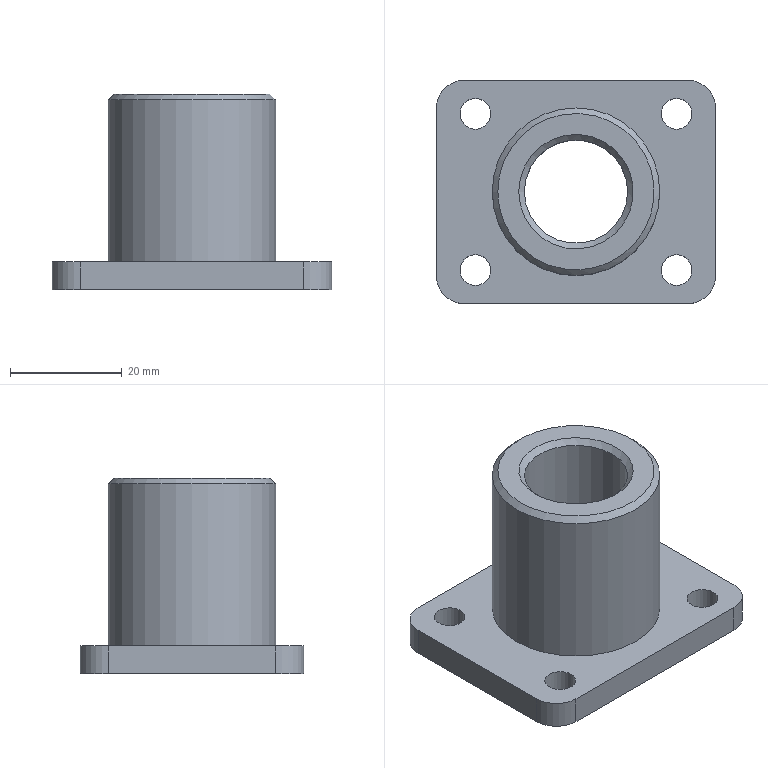NC program | NX | posted with a generic post | part box 50 x 40 x 35 mm
Whole program:
N10 G17 G21 G94 G90
(PLANAR_MILL , TOOL : D50面刀)
N12 T01 M6
N14 G53
N16 G17 G0 G90 X70. Y0. S3500 M3
N18 G43 Z20. H1
N20 Z3.
N22 G94 G1 Z0. F800.
N24 X20.
N26 X-20.
N28 X-70.
N30 Z3.
N32 G0 Z20.
N34 M5
(DRILLING , TOOL : D10倒角刀)
N36 T04 M6
N38 G53
N40 G17 G0 G90 X0. Y0. S1600 M3
N42 G43 Z20. H4
N44 G94 G81 G99 Z-2. F200. R3.
N46 G80
N48 G0 X0. Y0. Z20.
N50 M5
(DRILLING_COPY , TOOL : 14钻头)
N52 T06 M6
N54 G53
N56 G17 G0 G90 X0. Y0. S1600 M3
N58 G43 Z20. H6
N60 G94 G83 G99 Z-45. F250. Q3. R3.
N62 G80
N64 G0 X0. Y0. Z20.
N66 M5
(ADAPTIVE_MILLING , TOOL : D14开粗)
N68 T02 M6
N70 G53
N72 G17 G0 G90 X-43.532 Y-17.942 S6500 M3
N74 G43 Z20. H2
N76 Z-33.
N78 G94 G1 X-43.382 Y-17.95 Z-33.937 F2000.
N80 X-43.232 Y-17.957 Z-34.308
N82 X-43.082 Y-17.965 Z-34.58
N84 X-42.932 Y-17.972 Z-34.8
N86 X-42.783 Y-17.98 Z-34.984
N88 X-42.633 Y-17.987 Z-35.142
N90 X-42.483 Y-17.995 Z-35.28
N92 X-42.333 Y-18.002 Z-35.4
N94 X-42.183 Y-18.01 Z-35.505
N96 X-42.034 Y-18.017 Z-35.598
N98 X-41.884 Y-18.025 Z-35.679
N100 X-41.734 Y-18.032 Z-35.75
N102 X-41.584 Y-18.04 Z-35.81
N104 X-41.434 Y-18.047 Z-35.862
N106 X-41.284 Y-18.055 Z-35.905
N108 X-41.135 Y-18.062 Z-35.939
N110 X-40.985 Y-18.07 Z-35.966
N112 X-40.835 Y-18.077 Z-35.985
N114 X-40.685 Y-18.085 Z-35.996
N116 X-40.535 Y-18.092 Z-36.
N118 X-38.453 Y-18.196
N120 G3 X-37.016 Y-17.149 R1.414
N122 X-36.533 Y-13.375 R17.149
N124 X-36.401 Y-2.488 R270.705
N126 G1 X-36.399 Y22.214
N128 G2 X-33.919 Y27.676 R7.639
N130 X-28.648 Y30.469 R11.883
N132 X-22.412 Y31.271 R29.823
N134 X-10.623 Y31.399 R316.83
N136 G1 X27.261
N138 G2 X32.676 Y28.913 R7.655
N140 X35.469 Y23.637 R11.894
N142 X36.27 Y17.401 R29.853
N144 X36.398 Y5.657 R316.189
N146 G1 X36.4 Y-22.222
N148 G2 X33.984 Y-27.622 R7.616
N150 X28.819 Y-30.426 R11.696
N152 X22.677 Y-31.259 R28.633
N154 X12.059 Y-31.397 R260.732
N156 G1 X7.199 Y-31.4
N158 X-27.357 Y-31.398
N160 G2 X-32.715 Y-28.887 R7.676
N162 X-35.484 Y-23.601 R11.904
N164 X-36.072 Y-17.398 R21.042
N166 G3 X-35.801 Y-0.643 R380.067
N168 G1 X-35.8 Y19.424
N170 G2 X-31.703 Y27.393 R9.863
N172 X-25.709 Y29.964 R15.167
N174 X-18.51 Y30.696 R41.381
N176 X-3.436 Y30.8 R566.596
N178 G1 X24.503 Y30.799
N180 G2 X32.399 Y26.689 R9.871
N182 X34.958 Y20.73 R15.166
N184 X35.689 Y13.667 R40.664
N186 X35.799 Y-1.452 R535.868
N188 G1 X35.798 Y-19.567
N190 G2 X31.669 Y-27.422 R9.856
N192 X25.619 Y-29.984 R15.272
N194 X18.733 Y-30.688 R41.045
N196 X3.839 Y-30.799 R521.569
N198 G1 X-24.566 Y-30.798
N200 G2 X-32.451 Y-26.629 R9.868
N202 X-34.921 Y-20.358 R14.123
N204 X-35.279 Y-14.21 R39.912
N206 G1 X-35.204 Y-1.629
N208 X-35.201 Y2.819
N210 X-35.198 Y17.129
N212 G2 X-29.584 Y27.185 R11.38
N214 X-23.213 Y29.461 R18.218
N216 X-15.822 Y30.101 R51.205
N218 X-0.748 Y30.199 R632.596
N220 G1 X22.118 Y30.197
N222 G2 X32.12 Y24.685 R11.369
N224 X34.461 Y18.205 R18.106
N226 X35.1 Y10.814 R51.212
N228 X35.198 Y-3.765 R609.071
N230 G1 X35.197 Y-17.137
N232 G2 X29.715 Y-27.106 R11.346
N234 X23.371 Y-29.432 R17.945
N236 X15.803 Y-30.101 R50.392
N238 X0.728 Y-30.199 R636.552
N240 G1 X-22.137 Y-30.197
N242 G2 X-29.689 Y-27.53 R11.298
N244 X-33.537 Y-21.352 R13.017
N246 X-34.524 Y-14.782 R27.012
N248 X-34.619 Y-9.113 R151.751
N250 G1 X-34.613 Y11.532
N252 G2 X-34.531 Y16.689 R81.752
N254 X-28.342 Y26.506 R12.298
N256 X-21.572 Y28.845 R19.765
N258 X-13.326 Y29.509 R57.924
N260 X2.333 Y29.598 R787.319
N262 G1 X19.823 Y29.597
N264 G2 X25.174 Y28.771 R14.963
N266 X31.806 Y22.806 R12.578
N268 X33.943 Y15.962 R21.019
N270 X34.519 Y7.888 R64.124
N272 X34.598 Y-7.502 R831.686
N274 X34.564 Y-16.147 R327.966
N276 X28.33 Y-26.513 R12.319
N278 X21.544 Y-28.849 R19.837
N280 X13.658 Y-29.5 R56.548
N282 X-2.272 Y-29.598 R720.089
N284 G1 X-19.887 Y-29.597
N286 G2 X-25.275 Y-28.734 R14.703
N288 X-31.746 Y-22.661 R12.17
N290 X-33.576 Y-16.195 R20.188
N292 X-33.98 Y-8.83 R65.396
N294 G1 X-34.018 Y1.79
N296 G2 X-33.983 Y14.134 R697.678
N298 X-32.42 Y20.547 R14.428
N300 X-26.17 Y26.39 R13.695
N302 X-19.14 Y28.379 R23.417
N304 X-10.523 Y28.927 R74.411
N306 X4.867 Y28.998 R856.888
N308 G1 X17.797 Y28.997
N310 G2 X22.97 Y28.434 R19.245
N312 X30.83 Y22.215 R13.07
N314 X33.178 Y15.398 R20.771
N316 X33.878 Y7.425 R56.219
N318 X33.997 Y-8.054 R594.164
N320 X33.944 Y-14.753 R157.733
N322 X31.33 Y-22.25 R13.389
N324 X24.759 Y-26.999 R14.73
N326 X17.566 Y-28.567 R27.873
N328 X8.037 Y-28.962 R109.8
N330 G1 X-4.923 Y-28.998
N332 X-17.861 Y-28.996
N334 G2 X-23.031 Y-28.414 R18.708
N336 X-30.723 Y-22.081 R12.66
N338 X-32.828 Y-15.322 R20.451
N340 X-33.353 Y-7.515 R62.314
N342 X-33.387 Y12.505 R865.955
N344 X-32.16 Y18.645 R16.477
N346 X-29.105 Y23.006 R13.34
N348 G1 X-28.591 Y23.592
N350 X-27.396 Y24.64
N352 X-26.074 Y25.523
N354 X-24.649 Y26.225
N356 G2 X-17.453 Y27.846 R30.063
N358 X-7.75 Y28.344 R98.035
N360 X7.01 Y28.397 R895.492
N362 X17.76 Y28.363 R532.958
N364 X24.045 Y26.97 R15.784
N366 X27.947 Y24.157 R13.343
N368 G1 X28.592 Y23.591
N370 X29.64 Y22.396
N372 X30.523 Y21.074
N374 X31.225 Y19.649
N376 G2 X32.845 Y12.452 R30.107
N378 X33.339 Y3.019 R96.348
N380 X33.365 Y-12.68 R616.08
N382 X32.045 Y-18.888 R15.996
N384 X29.138 Y-22.968 R13.332
N386 G1 X28.591 Y-23.592
N388 X27.396 Y-24.64
N390 X26.074 Y-25.523
N392 X24.649 Y-26.225
N394 G2 X17.452 Y-27.845 R30.114
N396 X8.019 Y-28.339 R96.322
N398 X-7.011 Y-28.397 R888.753
N400 X-17.665 Y-28.366 R632.314
N402 X-23.661 Y-27.115 R15.692
N404 X-27.164 Y-24.795 R13.199
N406 G1 X-27.397 Y-24.639
N408 X-28.592 Y-23.591
N410 X-29.64 Y-22.396
N412 X-30.523 Y-21.074
N414 X-31.225 Y-19.649
N416 X-31.736 Y-18.144
N418 G2 X-32.417 Y-13.231 R34.125
N420 X-32.793 Y-2.44 R141.368
N422 X-32.796 Y11.145 R674.758
N424 X-32.076 Y16.121 R21.454
N426 G1 X-32.046 Y16.587
N428 X-31.736 Y18.146
N430 X-31.225 Y19.65
N432 X-30.522 Y21.076
N434 X-29.639 Y22.397
N436 X-28.591 Y23.592
N438 X-27.396 Y24.64
N440 X-26.074 Y25.523
N442 X-24.649 Y26.225
N444 X-23.144 Y26.736
N446 X-21.585 Y27.046
N448 G2 X-11.975 Y27.611 R540.608
N450 X3.953 Y27.795 R466.882
N452 X16.142 Y27.778 R845.082
N454 X21.076 Y27.079 R22.273
N456 G1 X21.587 Y27.046
N458 X23.146 Y26.736
N460 X24.65 Y26.225
N462 X26.076 Y25.522
N464 X27.397 Y24.639
N466 X27.972 Y24.134
N468 X27.397 Y24.639
N470 X26.076 Y25.522
N472 X24.65 Y26.225
N474 X23.146 Y26.736
N476 X21.587 Y27.046
N478 G3 X11.266 Y27.43 R117.228
N480 G1 X8.026 Y27.435
N482 X-16.089
N484 G2 X-17.302 Y28.138 R1.401
N486 X-17.235 Y29.638 Z-35.943 R1.408
N488 G1 X-16.551 Y30.616 Z-35.9
N490 X-16.015 Y31.382 F15000.
N492 G3 X-17.707 Y33.474 R1.4
N494 G1 X-18.122 Y33.301
N496 X-18.531 Y33.115
N498 G3 X-19.012 Y32.659 R1.417
N500 G1 X-20.324 Y30.628
N502 X-21.218 Y29.234 Z-35.96 F2000.
N504 G3 X-21.341 Y28.15 Z-36. R1.4
N506 X-20. Y27.15 R1.4
N508 G1 X20.
N510 X21.587 Y27.046
N512 X23.146 Y26.736
N514 X24.65 Y26.225
N516 X26.076 Y25.522
N518 X27.397 Y24.639
N520 X28.592 Y23.591
N522 X29.64 Y22.396
N524 X30.523 Y21.074
N526 X31.225 Y19.649
N528 X31.736 Y18.144
N530 X32.046 Y16.585
N532 G2 X32.612 Y6.926 R534.812
N534 X32.778 Y-11.037 R470.757
N536 X32.08 Y-16.061 R21.138
N538 G1 X32.046 Y-16.587
N540 X31.736 Y-18.146
N542 X31.225 Y-19.65
N544 X30.522 Y-21.076
N546 X29.639 Y-22.397
N548 X29.134 Y-22.972
N550 X29.639 Y-22.397
N552 X30.522 Y-21.076
N554 X31.225 Y-19.65
N556 X31.736 Y-18.146
N558 X32.046 Y-16.587
N560 G3 X32.422 Y-5.875 R116.901
N562 G1 X32.42 Y8.685
N564 X32.15 Y10.705
N566 Y15.
N568 Y-15.
N570 X32.046 Y-16.587
N572 X31.736 Y-18.146
N574 X31.225 Y-19.65
N576 X30.522 Y-21.076
N578 X29.639 Y-22.397
N580 X28.591 Y-23.592
N582 X27.396 Y-24.64
N584 X26.074 Y-25.523
N586 X24.649 Y-26.225
N588 X23.144 Y-26.736
N590 X21.585 Y-27.046
N592 G2 X12.052 Y-27.607 R563.562
N594 X-2.796 Y-27.793 R431.408
N596 X-16.045 Y-27.78 R944.863
N598 X-20.979 Y-27.086 R21.1
N600 G1 X-21.587 Y-27.046
N602 X-23.146 Y-26.736
N604 X-24.65 Y-26.225
N606 X-26.076 Y-25.522
N608 X-27.198 Y-24.772
N610 X-26.076 Y-25.522
N612 X-24.65 Y-26.225
N614 X-23.146 Y-26.736
N616 X-21.587 Y-27.046
N618 G3 X-11.191 Y-27.43 R117.669
N620 G1 X-7.771 Y-27.435
N622 X12.821 Y-27.433
N624 G2 X15.273 Y-27.15 R127.771
N626 G1 X20.
N628 X-20.
N630 X-21.587 Y-27.046
N632 X-23.146 Y-26.736
N634 X-24.65 Y-26.225
N636 X-26.076 Y-25.522
N638 X-27.397 Y-24.639
N640 X-28.592 Y-23.591
N642 X-29.64 Y-22.396
N644 X-30.523 Y-21.074
N646 X-31.225 Y-19.649
N648 X-31.736 Y-18.144
N650 X-32.046 Y-16.585
N652 X-32.15 Y-15.
N654 Y15.
N656 X-32.076 Y16.123
N658 G3 X-33.218 Y17.604 R1.414
N660 G1 X-35.305 Y18.008
N662 X-35.452 Y18.037 Z-35.996
N664 X-35.599 Y18.065 Z-35.985
N666 X-35.746 Y18.094 Z-35.966
N668 X-35.894 Y18.123 Z-35.939
N670 X-36.041 Y18.151 Z-35.905
N672 X-36.188 Y18.18 Z-35.862
N674 X-36.335 Y18.208 Z-35.81
N676 X-36.483 Y18.237 Z-35.75
N678 X-36.63 Y18.265 Z-35.679
N680 X-36.777 Y18.294 Z-35.598
N682 X-36.924 Y18.322 Z-35.505
N684 X-37.072 Y18.351 Z-35.4
N686 X-37.219 Y18.38 Z-35.28
N688 X-37.366 Y18.408 Z-35.142
N690 X-37.513 Y18.437 Z-34.984
N692 X-37.661 Y18.465 Z-34.8
N694 X-37.808 Y18.494 Z-34.58
N696 X-37.955 Y18.522 Z-34.308
N698 X-38.102 Y18.551 Z-33.937
N700 X-38.25 Y18.579 Z-33.
N702 G0 Z20.
N704 X-38.7 Y-6.809
N706 Z-26.85
N708 G1 X-38.55 Y-6.813 Z-27.787
N710 X-38.4 Y-6.817 Z-28.158
N712 X-38.25 Y-6.82 Z-28.43
N714 X-38.1 Y-6.824 Z-28.65
N716 X-37.95 Y-6.828 Z-28.834
N718 X-37.801 Y-6.831 Z-28.992
N720 X-37.651 Y-6.835 Z-29.13
N722 X-37.501 Y-6.839 Z-29.25
N724 X-37.351 Y-6.842 Z-29.355
N726 X-37.201 Y-6.846 Z-29.448
N728 X-37.051 Y-6.85 Z-29.529
N730 X-36.901 Y-6.853 Z-29.6
N732 X-36.751 Y-6.857 Z-29.66
N734 X-36.601 Y-6.861 Z-29.712
N736 X-36.451 Y-6.864 Z-29.755
N738 X-36.301 Y-6.868 Z-29.789
N740 X-36.151 Y-6.872 Z-29.816
N742 X-36.001 Y-6.876 Z-29.835
N744 X-35.851 Y-6.879 Z-29.846
N746 X-35.701 Y-6.883 Z-29.85
N748 X-33.567 Y-6.935
N750 G3 X-32.182 Y-5.94 R1.414
N752 X-31.703 Y-2.49 R15.204
N754 X-31.554 Y6.597 R197.471
N756 G2 X-31.507 Y13.923 R215.71
N758 X-29.004 Y21.222 R13.259
N760 X-22.352 Y25.589 R11.949
N762 X-16.389 Y26.402 R28.443
N764 X-5.68 Y26.547 R250.999
N766 G1 X-0.775 Y26.55
N768 X17.579 Y26.548
N770 G2 X23.737 Y25.432 R15.506
N772 X30.547 Y17.518 R11.813
N774 X31.405 Y11.381 R27.801
N776 X31.547 Y0.627 R256.51
N778 G1 X31.549 Y-12.328
N780 G2 X30.778 Y-17.827 R16.712
N782 X22.452 Y-25.562 R11.825
N784 X16.311 Y-26.406 R28.272
N786 X5.648 Y-26.547 R257.185
N788 G1 X0.788 Y-26.55
N790 X-17.522 Y-26.548
N792 G2 X-23.474 Y-25.54 R15.778
N794 X-30.563 Y-17.452 R11.817
N796 X-31.399 Y-11.447 R27.928
N798 X-31.276 Y-5.091 R43.192
N800 G3 X-30.958 Y7.369 R191.883
N802 G2 X-30.866 Y12.894 R85.759
N804 X-28.861 Y19.36 R13.812
N806 X-22.748 Y24.212 R12.536
N808 X-16.349 Y25.607 R23.605
N810 X-7.718 Y25.928 R103.177
N812 G1 X2.677 Y25.949
N814 X15.312 Y25.948
N816 G2 X20.716 Y25.415 R21.701
N818 X28.899 Y18.494 R12.045
N820 X30.534 Y12.065 R21.292
N822 X30.92 Y3.573 R85.532
N824 X30.92 Y-11.926 R744.474
N826 X29.606 Y-18.001 R15.514
N828 X23.265 Y-23.998 R12.141
N830 X16.947 Y-25.545 R21.872
N832 X8.453 Y-25.921 R87.79
N834 G1 X-2.436 Y-25.949
N836 X-15.307 Y-25.948
N838 G2 X-20.711 Y-25.416 R21.734
N840 X-28.932 Y-18.416 R12.054
N842 X-30.569 Y-11.66 R21.66
N844 X-30.631 Y-5.32 R49.027
N846 G3 X-30.339 Y9.899 R434.182
N848 G2 X-29.53 Y15.444 R18.973
N850 X-23.102 Y22.781 R12.665
N852 X-16.311 Y24.779 R21.244
N854 X-8.097 Y25.291 R69.757
N856 X4.773 Y25.349 R787.252
N858 X15.492 Y25.314 R544.392
N860 X21.172 Y24.264 R16.888
N862 X27.869 Y17.933 R12.755
N864 X29.794 Y11.211 R21.534
N866 X30.293 Y3.041 R70.958
N868 X30.31 Y-10.594 R418.892
N870 X29.175 Y-16.391 R16.492
N872 X22.814 Y-22.925 R12.802
N874 X16.032 Y-24.816 R21.962
N876 X7.635 Y-25.299 R75.047
N878 X-4.785 Y-25.349 R790.412
N880 X-15.487 Y-25.314 R545.573
N882 X-21.167 Y-24.266 R16.912
N884 X-27.876 Y-17.915 R12.753
N886 X-29.811 Y-10.513 R20.615
N888 X-29.93 Y-3.497 R66.222
N890 G3 X-29.735 Y8.839 R999.429
N892 G2 X-28.851 Y14.463 R18.936
N894 X-22.272 Y21.946 R13.339
N896 X-15.333 Y24.08 R21.918
N898 X-6.72 Y24.677 R67.673
N900 X13.962 Y24.716 R869.82
N902 X19.537 Y23.819 R18.458
N904 X26.954 Y17.259 R13.335
N906 X29.076 Y10.367 R21.88
N908 X29.679 Y1.664 R67.715
N910 X29.695 Y-9.45 R249.339
N912 X28.513 Y-15.33 R16.713
N914 X21.982 Y-22.094 R13.478
N916 X14.963 Y-24.134 R22.694
N918 X6.031 Y-24.691 R74.436
N920 X-13.957 Y-24.716 R893.754
N922 X-19.576 Y-23.806 R18.421
N924 X-27.034 Y-17.093 R13.335
N926 X-29.013 Y-9.969 R20.714
N928 X-29.269 Y-2.103 R66.869
N930 X-29.112 Y8.223 R463.309
N932 X-27.896 Y14.235 R17.553
N934 X-21.222 Y21.276 R14.033
N936 X-13.971 Y23.462 R23.238
N938 X-4.863 Y24.076 R72.374
N940 X12.596 Y24.114 R676.558
N942 X18.44 Y23.19 R19.381
N944 X26.213 Y16.341 R13.911
N946 X28.436 Y9.151 R22.843
N948 X29.062 Y0.585 R67.693
N950 X29.069 Y-8.503 R148.851
N952 X27.68 Y-14.701 R16.587
N954 X20.951 Y-21.41 R14.141
N956 X13.712 Y-23.499 R23.864
N958 X4.692 Y-24.08 R75.191
N960 X-12.768 Y-24.108 R606.454
N962 X-18.687 Y-23.102 R18.717
N964 X-26.389 Y-15.94 R13.855
N966 X-28.312 Y-8.756 R22.18
N968 X-28.625 Y-0.532 R73.519
N970 X-28.488 Y7.476 R161.926
N972 X-26.951 Y13.914 R17.178
N974 X-20.04 Y20.708 R14.713
N976 X-12.638 Y22.857 R24.676
N978 X-3.529 Y23.467 R75.35
N980 X11.455 Y23.506 R465.588
N982 X17.431 Y22.547 R20.016
N984 X25.484 Y15.473 R14.418
N986 X27.762 Y8.25 R23.398
N988 X28.446 Y-0.447 R66.134
N990 X28.41 Y-7.959 R83.176
N992 X26.41 Y-14.904 R15.881
N994 X19.536 Y-20.942 R15.001
N996 X12.171 Y-22.921 R25.907
N998 X2.878 Y-23.479 R82.782
N1000 X-11.656 Y-23.499 R418.246
N1002 X-17.704 Y-22.449 R19.28
N1004 X-25.651 Y-15.028 R14.262
N1006 X-27.617 Y-7.714 R23.245
N1008 X-27.992 Y1.003 R77.179
N1010 X-27.77 Y7.611 R61.165
N1012 X-24.893 Y15.325 R15.649
N1014 X-17.828 Y20.611 R16.157
N1016 X-10.226 Y22.4 R29.144
N1018 X-0.253 Y22.894 R102.694
N1020 X10.726 Y22.881 R260.63
N1022 X17.021 Y21.699 R19.389
N1024 X24.84 Y14.499 R14.934
N1026 X27.123 Y7.222 R24.237
N1028 X27.846 Y-2.103 R68.436
N1030 X27.627 Y-8.302 R39.731
N1032 X19.63 Y-19.766 R14.85
N1034 X12.32 Y-22.104 R23.963
N1036 X3.266 Y-22.834 R66.633
N1038 X-10.547 Y-22.888 R302.39
N1040 X-16.769 Y-21.793 R19.901
N1042 X-24.828 Y-14.345 R14.596
N1044 X-26.903 Y-6.966 R23.637
N1046 X-27.353 Y2.737 R74.53
N1048 X-26.774 Y8.817 R28.301
N1050 X-18.893 Y19.03 R15.263
N1052 X-11.34 Y21.469 R24.443
N1054 X-2.288 Y22.219 R67.157
N1056 X9.703 Y22.265 R206.019
N1058 X16.213 Y21.008 R19.832
N1060 X24.049 Y13.848 R15.287
N1062 X26.494 Y6.194 R24.649
N1064 X27.125 Y-5.918 R59.091
N1066 X24.973 Y-13.28 R16.662
N1068 X17.967 Y-19.484 R15.785
N1070 X10.411 Y-21.612 R26.578
N1072 X1.033 Y-22.251 R79.484
N1074 X-9.653 Y-22.267 R202.031
N1076 X-15.996 Y-21.089 R20.04
N1078 X-24.109 Y-13.497 R14.965
N1080 X-26.209 Y-6.171 R24.205
N1082 X-26.566 Y5.1 R56.14
N1084 X-24.25 Y12.6 R17.201
N1086 X-16.923 Y18.917 R16.312
N1088 X-9.218 Y21.016 R27.8
N1090 X-5.591 Y21.403 R100.957
N1092 G1 X-4.484 Y21.691
N1094 X-2.265 Y22.034
N1096 X-0.084 Y22.15
N1098 G2 X3.673 Y21.898 R54.479
N1100 X9.54 Y21.623 R328.258
N1102 X16.355 Y19.916 R18.822
N1104 X23.64 Y12.496 R15.91
N1106 X25.952 Y4.67 R26.511
N1108 X26.453 Y-4.975 R47.583
N1110 X24.132 Y-12.704 R16.776
N1112 X16.982 Y-18.876 R16.209
N1114 X9.328 Y-20.997 R27.441
N1116 X5.609 Y-21.399 R88.474
N1118 G1 X4.445 Y-21.699
N1120 X2.233 Y-22.037
N1122 X-0.001 Y-22.15
N1124 G2 X-3.987 Y-21.883 R86.144
N1126 X-9.807 Y-21.6 R183.485
N1128 X-16.589 Y-19.784 R18.136
N1130 X-23.541 Y-12.372 R15.546
N1132 X-25.617 Y-4.714 R25.865
N1134 X-25.862 Y4.624 R42.833
N1136 X-22.94 Y12.756 R16.753
N1138 X-15.639 Y18.454 R17.028
N1140 X-8.842 Y20.316 R29.363
N1142 G1 X-6.658 Y21.126
N1144 X-5.569 Y21.409
N1146 X-6.658 Y21.126
N1148 G2 X-10.027 Y19.9 R64.799
N1150 G3 X-15.272 Y18.104 R41.184
N1152 X-22.352 Y12.509 R17.012
N1154 X-25.307 Y4.622 R17.22
N1156 X-24.387 Y-8.634 R35.987
N1158 X-20.459 Y-16.018 R18.01
N1160 X-12.121 Y-20.683 R15.615
N1162 X-6.588 Y-21.36 R35.88
N1164 G2 X-4.446 Y-21.699 R6.931
N1166 G1 X-2.355 Y-22.019
N1168 X-4.446 Y-21.699
N1170 G3 X-9.745 Y-20.521 R53.886
N1172 G2 X-16.035 Y-18.294 R20.022
N1174 X-22.686 Y-10.638 R16.154
N1176 X-24.675 Y-2.265 R26.777
N1178 X-24.287 Y5.75 R26.792
N1180 X-16.254 Y16.552 R16.199
N1182 X-12.36 Y18.361 R31.331
N1184 G1 X-10.778 Y19.351
N1186 X-8.84 Y20.305
N1188 X-10.778 Y19.351
N1190 G2 X-15.416 Y16.587 R92.283
N1192 G3 X-21.311 Y11.201 R18.071
N1194 X-24.177 Y2.854 R18.017
N1196 X-22.704 Y-9.241 R27.595
N1198 X-16.561 Y-17.22 R16.411
N1200 X-10.296 Y-19.886 R19.858
N1202 G1 X-8.99 Y-20.229
N1204 X-8.711 Y-20.365
N1206 X-6.612 Y-21.14
N1208 X-8.711 Y-20.365
N1210 G3 X-12.745 Y-18.496 R109.92
N1212 G2 X-20.598 Y-11.446 R17.49
N1214 X-23.377 Y-2.434 R22.404
N1216 X-22.631 Y6.249 R21.827
N1218 X-16.546 Y14.732 R17.
N1220 G3 X-16.081 Y15.232 R7.026
N1222 G1 X-14.456 Y16.782
N1224 X-12.682 Y18.16
N1226 X-14.456 Y16.782
N1228 X-16.081 Y15.232
N1230 X-18.643 Y12.313
N1232 G3 X-22.97 Y0.758 R18.678
N1234 X-20.69 Y-10.139 R22.38
N1236 X-13.622 Y-17.431 R17.636
N1238 G1 X-12.621 Y-18.203
N1240 X-10.72 Y-19.383
N1242 X-10.235 Y-19.62
N1244 X-10.72 Y-19.383
N1246 X-12.621 Y-18.203
N1248 X-14.392 Y-16.837
N1250 X-16.017 Y-15.299
N1252 G2 X-18.622 Y-12.026 R29.254
N1254 X-21.987 Y2.452 R21.668
N1256 G1 X-21.902 Y3.303
N1258 X-21.455 Y5.504
N1260 X-20.788 Y7.648
N1262 X-19.906 Y9.714
N1264 X-18.82 Y11.68
N1266 X-17.541 Y13.525
N1268 X-16.78 Y14.415
N1270 X-17.541 Y13.525
N1272 X-18.82 Y11.68
N1274 X-19.906 Y9.714
N1276 X-20.788 Y7.648
N1278 X-21.455 Y5.504
N1280 X-21.902 Y3.303
N1282 X-22.124 Y1.065
N1284 X-22.109 Y-1.27
N1286 X-21.886 Y-3.412
N1288 X-21.428 Y-5.611
N1290 X-20.749 Y-7.752
N1292 X-19.858 Y-9.813
N1294 X-18.762 Y-11.774
N1296 X-17.479 Y-13.606
N1298 X-16.017 Y-15.299
N1300 X-14.392 Y-16.837
N1302 X-12.621 Y-18.203
N1304 X-10.72 Y-19.383
N1306 X-8.711 Y-20.365
N1308 X-6.612 Y-21.14
N1310 X-4.446 Y-21.699
N1312 X-2.235 Y-22.037
N1314 X-0.001 Y-22.15
N1316 X2.233 Y-22.037
N1318 X4.445 Y-21.699
N1320 G2 X9.358 Y-20.646 R44.229
N1322 G3 X16.178 Y-18.69 R29.703
N1324 X23.405 Y-12.656 R16.168
N1326 X25.89 Y-5.105 R17.182
N1328 X24.732 Y8.276 R38.542
N1330 X20.888 Y15.654 R19.058
N1332 X12.039 Y20.708 R15.9
N1334 X6.414 Y21.37 R37.422
N1336 G1 X5.445 Y21.441
N1338 X4.258 Y21.737
N1340 X2.387 Y22.008
N1342 X4.258 Y21.737
N1344 G3 X10.214 Y20.431 R78.094
N1346 G2 X16.923 Y17.789 R19.024
N1348 X23.08 Y10.224 R16.892
N1350 X25.151 Y1.547 R28.923
N1352 X24.901 Y-6.298 R27.609
N1354 X16.744 Y-17.33 R15.715
N1356 X10.072 Y-19.736 R26.61
N1358 G3 X8.709 Y-20.366 R10.83
N1360 G1 X6.611 Y-21.14
N1362 X6.219 Y-21.242
N1364 X6.611 Y-21.14
N1366 X8.709 Y-20.366
N1368 G2 X12.733 Y-18.658 R30.957
N1370 G3 X18.762 Y-15.359 R21.779
N1372 X24.412 Y-5.722 R15.921
N1374 X24.454 Y3.505 R27.923
N1376 X21.865 Y11.523 R23.753
N1378 X12.504 Y19.246 R16.508
N1380 X8.952 Y20.243 R48.126
N1382 G1 X8.573 Y20.424
N1384 X6.449 Y21.19
N1386 X8.573 Y20.424
N1388 G3 X12.598 Y18.592 R89.762
N1390 G2 X20.019 Y12.641 R18.181
N1392 X23.479 Y4.335 R21.496
N1394 X23.631 Y-5.278 R24.814
N1396 X16.164 Y-15.98 R16.069
N1398 X13.756 Y-17.327 R42.039
N1400 G1 X12.619 Y-18.204
N1402 X10.719 Y-19.384
N1404 X10.153 Y-19.66
N1406 X10.719 Y-19.384
N1408 X12.619 Y-18.204
N1410 G2 X16.645 Y-15.197 R181.353
N1412 G3 X23.37 Y-3.186 R16.977
N1414 X21.159 Y9.691 R23.837
N1416 X13.416 Y17.593 R18.139
N1418 G1 X12.532 Y18.264
N1420 X10.608 Y19.445
N1422 X10.202 Y19.64
N1424 X10.608 Y19.445
N1426 X12.532 Y18.264
N1428 X14.327 Y16.893
N1430 G2 X18.138 Y12.9 R32.855
N1432 X22.293 Y-4.449 R22.006
N1434 X18.513 Y-12.13 R16.501
N1436 G1 X17.478 Y-13.607
N1438 X16.016 Y-15.301
N1440 X14.284 Y-16.92
N1442 X16.016 Y-15.301
N1444 X17.478 Y-13.607
N1446 X18.761 Y-11.775
N1448 G3 X20.662 Y-8.035 R29.665
N1450 X22.121 Y0.163 R20.043
N1452 G1 Y1.14
N1454 X21.89 Y3.386
N1456 X21.431 Y5.597
N1458 X20.75 Y7.75
N1460 X19.853 Y9.822
N1462 X18.75 Y11.793
N1464 X17.452 Y13.64
N1466 X15.972 Y15.346
N1468 X17.452 Y13.64
N1470 X18.75 Y11.793
N1472 X19.853 Y9.822
N1474 X20.75 Y7.75
N1476 X21.431 Y5.597
N1478 X21.89 Y3.386
N1480 X22.121 Y1.14
N1482 X22.122 Y-1.118
N1484 X21.893 Y-3.365
N1486 X21.436 Y-5.577
N1488 X20.757 Y-7.73
N1490 X19.862 Y-9.804
N1492 G3 X20.25 Y-11.445 R1.414
N1494 G1 X22.068 Y-12.977
N1496 X22.183 Y-13.074 Z-29.846
N1498 X22.297 Y-13.171 Z-29.835
N1500 X22.412 Y-13.267 Z-29.816
N1502 X22.527 Y-13.364 Z-29.789
N1504 X22.642 Y-13.46 Z-29.755
N1506 X22.756 Y-13.557 Z-29.712
N1508 X22.871 Y-13.654 Z-29.66
N1510 X22.986 Y-13.75 Z-29.6
N1512 X23.1 Y-13.847 Z-29.529
N1514 X23.215 Y-13.944 Z-29.448
N1516 X23.33 Y-14.04 Z-29.355
N1518 X23.445 Y-14.137 Z-29.25
N1520 X23.559 Y-14.234 Z-29.13
N1522 X23.674 Y-14.33 Z-28.992
N1524 X23.789 Y-14.427 Z-28.834
N1526 X23.904 Y-14.524 Z-28.65
N1528 X24.018 Y-14.62 Z-28.43
N1530 X24.133 Y-14.717 Z-28.158
N1532 X24.248 Y-14.813 Z-27.787
N1534 X24.362 Y-14.91 Z-26.85
N1536 G0 Z20.
(HOLE_MILLING , TOOL : D14开粗)
N1538 X0. Y0. S3500
N1540 Z2.
N1542 G3 X1.125 Y-1.125 R1.125 F500.
N1544 X2.25 Y0. R1.125
N1546 X2.25 Y0. Z1. I-2.25 J0.
N1548 X2.25 Y0. Z0. I-2.25 J0.
N1550 X2.25 Y0. Z-1. I-2.25 J0.
N1552 X2.25 Y0. Z-2. I-2.25 J0.
N1554 X2.25 Y0. Z-3. I-2.25 J0.
N1556 X2.25 Y0. Z-4. I-2.25 J0.
N1558 X2.25 Y0. Z-5. I-2.25 J0.
N1560 X2.25 Y0. Z-6. I-2.25 J0.
N1562 X2.25 Y0. Z-7. I-2.25 J0.
N1564 X2.25 Y0. Z-8. I-2.25 J0.
N1566 X2.25 Y0. Z-9. I-2.25 J0.
N1568 X2.25 Y0. Z-10. I-2.25 J0.
N1570 X2.25 Y0. Z-11. I-2.25 J0.
N1572 X2.25 Y0. Z-12. I-2.25 J0.
N1574 X2.25 Y0. Z-13. I-2.25 J0.
N1576 X2.25 Y0. Z-14. I-2.25 J0.
N1578 X2.25 Y0. Z-15. I-2.25 J0.
N1580 X2.25 Y0. Z-16. I-2.25 J0.
N1582 X2.25 Y0. Z-17. I-2.25 J0.
N1584 X2.25 Y0. Z-18. I-2.25 J0.
N1586 X2.25 Y0. Z-19. I-2.25 J0.
N1588 X2.25 Y0. Z-20. I-2.25 J0.
N1590 X2.25 Y0. Z-21. I-2.25 J0.
N1592 X2.25 Y0. Z-22. I-2.25 J0.
N1594 X2.25 Y0. Z-23. I-2.25 J0.
N1596 X2.25 Y0. Z-24. I-2.25 J0.
N1598 X2.25 Y0. Z-25. I-2.25 J0.
N1600 X2.25 Y0. Z-26. I-2.25 J0.
N1602 X2.25 Y0. Z-27. I-2.25 J0.
N1604 X2.25 Y0. Z-28. I-2.25 J0.
N1606 X2.25 Y0. Z-29. I-2.25 J0.
N1608 X2.25 Y0. Z-30. I-2.25 J0.
N1610 X2.25 Y0. Z-31. I-2.25 J0.
N1612 X2.25 Y0. Z-32. I-2.25 J0.
N1614 X2.25 Y0. Z-33. I-2.25 J0.
N1616 X2.25 Y0. Z-34. I-2.25 J0.
N1618 X2.25 Y0. Z-35. I-2.25 J0.
N1620 X2.25 Y0. Z-36. I-2.25 J0.
N1622 X2.25 Y0. Z-37. I-2.25 J0.
N1624 X2.25 Y0. Z-38. I-2.25 J0.
N1626 X0. Y2.25 R2.25
N1628 X2.25 Y0. R-2.25
N1630 X1.125 Y1.125 R1.125
N1632 X0. Y0. R1.125
N1634 G0 Z20.
(PLANAR_MILL_2 , TOOL : D14开粗)
N1636 X-0.75 Y1.
N1638 Z-34.
N1640 G1 Z-36. F300.
N1642 X-1.25
N1644 G3 X-2.25 Y0. R1.
N1646 X0. Y-2.25 R2.25
N1648 X-2.25 Y0. R-2.25
N1650 X-1.25 Y-1. R1.
N1652 G1 X-0.75
N1654 Z-34.
N1656 G0 Z20.
N1658 M5
(DRILLING_1 , TOOL : D10倒角刀)
N1660 T04 M6
N1662 G53
N1664 G17 G0 G90 X-18. Y14. S1600 M3
N1666 G43 Z20. H4
N1668 G94 G81 G98 Z-32.75 F250. R-27.
N1670 X18.
N1672 Y-14.
N1674 X-18.
N1676 G80
N1678 G0 X-18. Y-14. Z20.
(PLANAR_MILL_1 , TOOL : D10倒角刀)
N1680 X19. Y2. S3500
N1682 Z-1.
N1684 G1 Z-3. F1000.
N1686 G3 X17. Y0. R2.
N1688 G2 X0. Y-17. R17.
N1690 X17. Y0. R-17.
N1692 G3 X19. Y-2. R2.
N1694 G1 Z-1.
N1696 G0 Z20.
(PLANAR_MILL_1_COPY , TOOL : D10倒角刀)
N1698 X-5.07 Y2.
N1700 Z-1.
N1702 G1 Z-3.
N1704 X-5.45
N1706 G3 X-7.45 Y0. R2.
N1708 X0. Y-7.45 R7.45
N1710 X-7.45 Y0. R-7.45
N1712 X-5.45 Y-2. R2.
N1714 G1 X-5.07
N1716 Z-1.
N1718 G0 Z20.
(PLANAR_MILL_1_COPY_COPY , TOOL : D10倒角刀)
N1720 X-28.9
N1722 Z-30.
N1724 G1 Z-32.
N1726 G3 X-26.9 Y0. R2.
N1728 G1 Y15.
N1730 G2 X-20. Y21.9 R6.9
N1732 G1 X20.
N1734 G2 X26.9 Y15. R6.9
N1736 G1 Y-15.
N1738 G2 X20. Y-21.9 R6.9
N1740 G1 X-20.
N1742 G2 X-26.9 Y-15. R6.9
N1744 G1 Y0.
N1746 G3 X-28.9 Y2. R2.
N1748 G1 Z-30.
N1750 G0 Z20.
N1752 M5
(DRILLING_1_COPY , TOOL : 5.5钻头)
N1754 T05 M6
N1756 G53
N1758 G17 G0 G90 X-18. Y14. S2000 M3
N1760 G43 Z20. H5
N1762 G94 G81 G98 Z-38. F150. R-27.
N1764 X18.
N1766 Y-14.
N1768 X-18.
N1770 G80
N1772 G0 X-18. Y-14. Z20.
N1774 M5
(THREAD_MILLING , TOOL : D12-1.5)
N1776 T07 M6
N1778 G53
N1780 G17 G0 G90 X0. Y0. S2000 M3
N1782 G43 Z20. H7
N1784 Z-38.244
N1786 G41 G94 G1 X-0.297 Y-0.043 F200. D7
N1788 G3 X-0.356 Y-0.617 Z-38. R0.316
N1790 X-0.356 Y-0.617 Z-36.5 I0.356 J0.617
N1792 X-0.356 Y-0.617 Z-35. I0.356 J0.617
N1794 X-0.356 Y-0.617 Z-33.5 I0.356 J0.617
N1796 X-0.356 Y-0.617 Z-32. I0.356 J0.617
N1798 X-0.356 Y-0.617 Z-30.5 I0.356 J0.617
N1800 X-0.356 Y-0.617 Z-29. I0.356 J0.617
N1802 X-0.356 Y-0.617 Z-27.5 I0.356 J0.617
N1804 X-0.356 Y-0.617 Z-26. I0.356 J0.617
N1806 X-0.356 Y-0.617 Z-24.5 I0.356 J0.617
N1808 X-0.356 Y-0.617 Z-23. I0.356 J0.617
N1810 X-0.356 Y-0.617 Z-21.5 I0.356 J0.617
N1812 X-0.356 Y-0.617 Z-20. I0.356 J0.617
N1814 X-0.356 Y-0.617 Z-18.5 I0.356 J0.617
N1816 X-0.356 Y-0.617 Z-17. I0.356 J0.617
N1818 X-0.356 Y-0.617 Z-15.5 I0.356 J0.617
N1820 X-0.356 Y-0.617 Z-14. I0.356 J0.617
N1822 X-0.356 Y-0.617 Z-12.5 I0.356 J0.617
N1824 X-0.356 Y-0.617 Z-11. I0.356 J0.617
N1826 X-0.356 Y-0.617 Z-9.5 I0.356 J0.617
N1828 X-0.356 Y-0.617 Z-8. I0.356 J0.617
N1830 X-0.356 Y-0.617 Z-6.5 I0.356 J0.617
N1832 X-0.356 Y-0.617 Z-5. I0.356 J0.617
N1834 X-0.356 Y-0.617 Z-3.5 I0.356 J0.617
N1836 X-0.356 Y-0.617 Z-2. I0.356 J0.617
N1838 X-0.356 Y-0.617 Z-0.5 I0.356 J0.617
N1840 X-0.356 Y-0.617 Z1. I0.356 J0.617
N1842 X0.111 Y-0.279 Z1.244 R0.316
N1844 G40
N1846 G1 X0. Y0.
N1848 G0 Z20.
N1850 M5
(PLANAR_MILL_3 , TOOL : D16精光)
N1852 T03 M6
N1854 G53
N1856 G17 G0 G90 X-18. Y-30. S3500 M3
N1858 G43 Z20. H3
N1860 Z-34.
N1862 G94 G1 Z-36. F600.
N1864 G3 X-20. Y-28. R2.
N1866 G2 X-33. Y-15. R13.
N1868 G1 Y15.
N1870 G2 X-20. Y28. R13.
N1872 G1 X20.
N1874 G2 X33. Y15. R13.
N1876 G1 Y-15.
N1878 G2 X20. Y-28. R13.
N1880 G1 X-20.
N1882 G3 X-22. Y-30. R2.
N1884 G1 Z-34.
N1886 G0 Z20.
(PLANAR_MILL_3_COPY , TOOL : D16精光)
N1888 X-28. Y-2.
N1890 Z-28.
N1892 G1 Z-30.
N1894 G3 X-26. Y0. R2.
N1896 G2 X0. Y26. R26.
N1898 X-26. Y0. R-26.
N1900 G3 X-28. Y2. R2.
N1902 G1 X-25. Y-2.
N1904 G3 X-23. Y0. R2.
N1906 G2 X0. Y23. R23.
N1908 X-23. Y0. R-23.
N1910 G3 X-25. Y2. R2.
N1912 G1 X-27.928
N1914 Z-28.
N1916 G0 Z20.
(PLANAR_MILL_3_COPY_COPY , TOOL : D16精光)
N1918 X-25.985 Y-1.826
N1920 Z-27.995
N1922 G1 Z-29.995
N1924 G41 X-25. Y-2. D3
N1926 G3 X-23. Y0. R2.
N1928 G2 X0. Y23. R23.
N1930 X-23. Y0. R-23.
N1932 G3 X-25. Y2. R2.
N1934 G40
N1936 G1 X-25.985 Y1.826
N1938 Z-27.995
N1940 G0 Z20.
N1942 M5
(PLANAR_MILL_COPY , TOOL : D50面刀)
N1944 T01 M6
N1946 G53
N1948 G17 G0 G90 X70. Y0. S3500 M3
N1950 G43 Z20. H1
N1952 Z3.
N1954 G94 G1 Z0. F800.
N1956 X20.
N1958 X-20.
N1960 X-70.
N1962 Z3.
N1964 G0 Z20.
N1966 M5
(PLANAR_MILL_4 , TOOL : D10倒角刀)
N1968 T04 M6
N1970 G53
N1972 G17 G0 G90 X28.5 Y2. S3500 M3
N1974 G43 Z20. H4
N1976 Z0.5
N1978 G94 G1 Z-1.5 F800.
N1980 G3 X26.5 Y0. R2.
N1982 G1 Y-15.
N1984 G2 X20. Y-21.5 R6.5
N1986 G1 X-20.
N1988 G2 X-26.5 Y-15. R6.5
N1990 G1 Y15.
N1992 G2 X-20. Y21.5 R6.5
N1994 G1 X20.
N1996 G2 X26.5 Y15. R6.5
N1998 G1 Y0.
N2000 G3 X28.5 Y-2. R2.
N2002 G1 Z0.5
N2004 G0 Z20.
(PLANAR_MILL_4_COPY , TOOL : D10倒角刀)
N2006 X5.07
N2008 Z-1.
N2010 G1 Z-3.
N2012 X5.45
N2014 G3 X7.45 Y0. R2.
N2016 X0. Y7.45 R7.45
N2018 X7.45 Y0. R-7.45
N2020 X5.45 Y2. R2.
N2022 G1 X5.07
N2024 Z-1.
N2026 G0 Z20.
(DRILLING_2 , TOOL : D10倒角刀)
N2028 X-18. Y14. S2000
N2030 G81 G99 Z-2.75 F250. R3.
N2032 X18.
N2034 Y-14.
N2036 X-18.
N2038 G80
N2040 G0 X-18. Y-14. Z20.
N2042 M5
N2044 M2